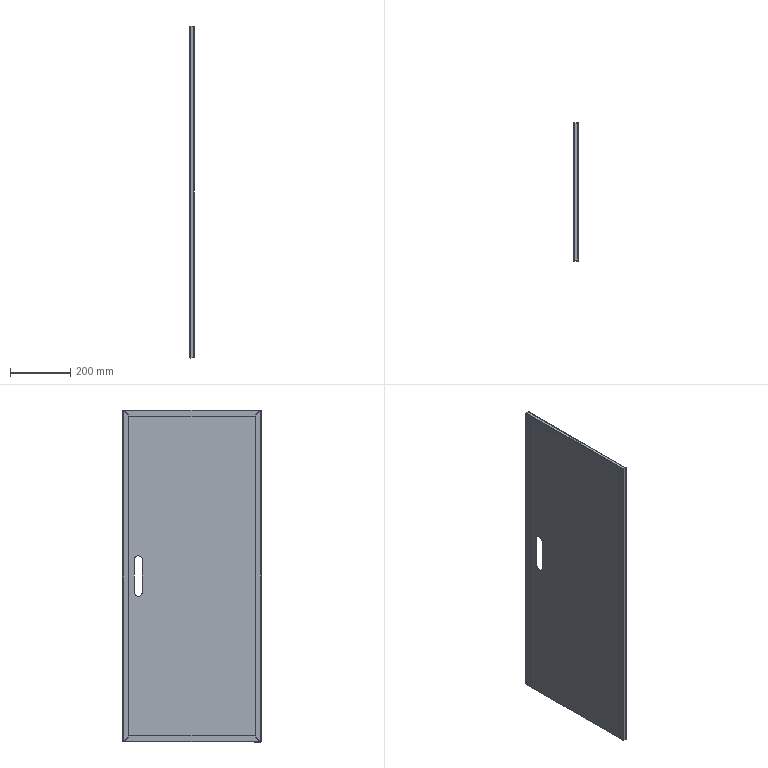Part | STEP file | MEN5-2 | 1 solid | 79 faces | box 15 x 461 x 1106 mm | volume 897799 mm3 | plane 44 | cylinder 27 | spline 8 | commonest cylinder face diameters 6 x16 3 x8 27 x3